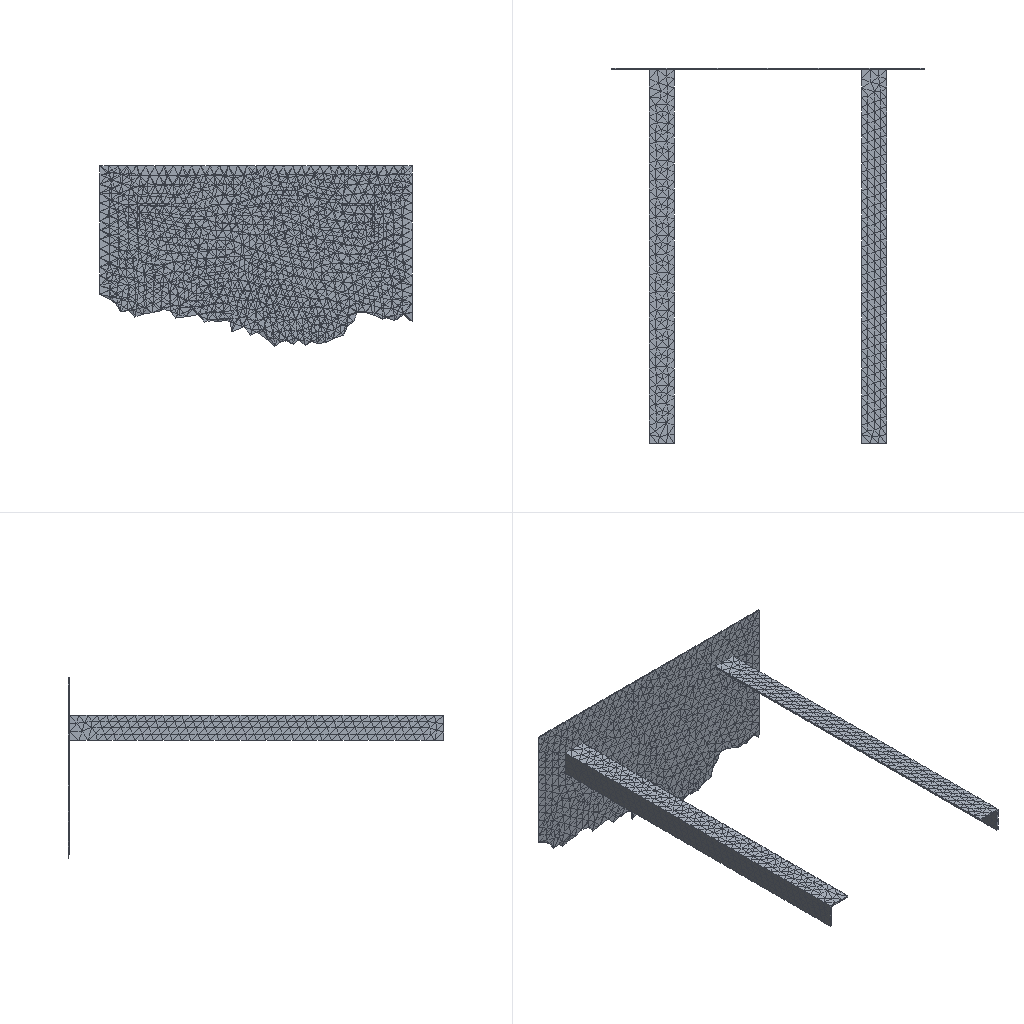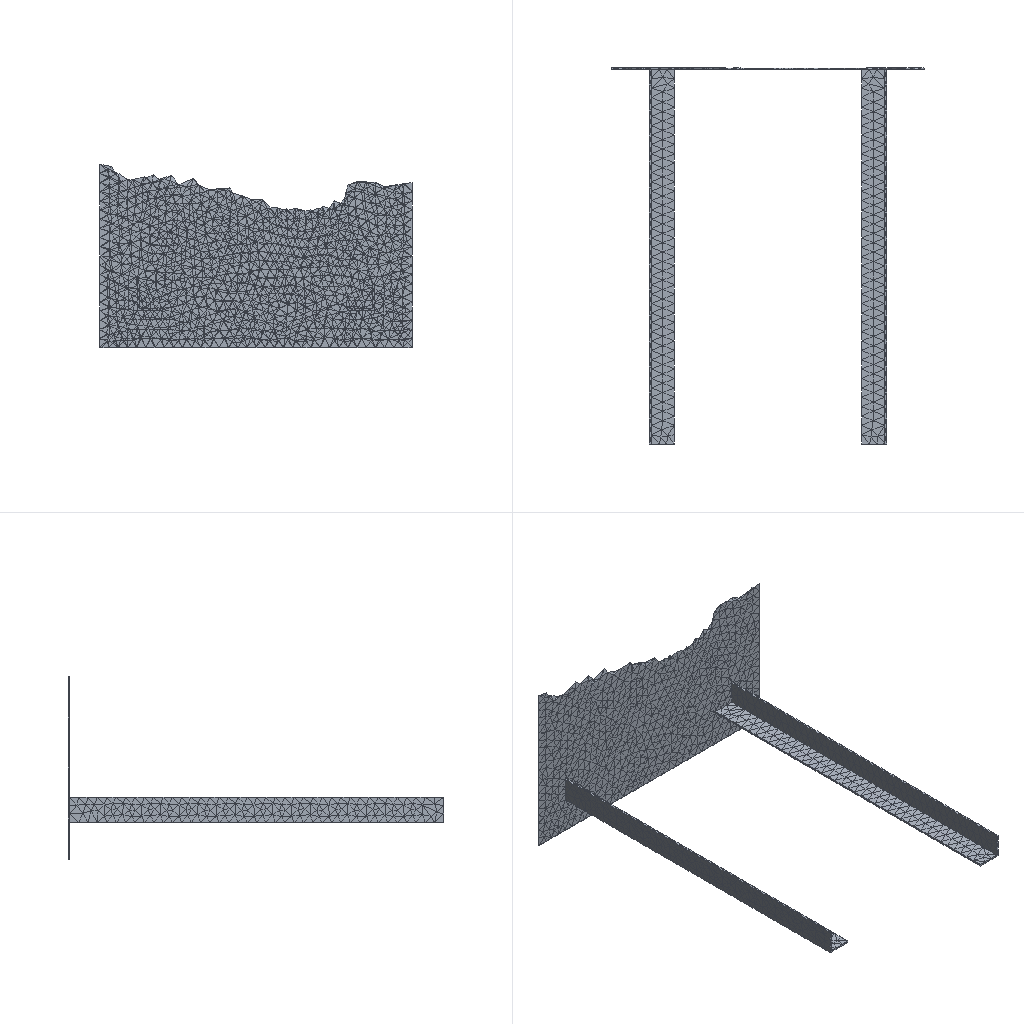Simulation study | ansys mapdl
Set-up summary:
category,name,step,type,value,unit,region
solver,ansys_mapdl
solver,version,,,21.1
solver,version,,,21.1
solver,version,,,21.1
units,MPA,,stated
analysis,deck,,modal,modal
load_step,requested,,,1
analysis,nlgeom,,,False
mesh,nodes,,,27244
mesh,elements,,,12925
element_type,ANSYS 187 (type 1),,solid,12925
load,load commands in deck,,count,0
bc,support commands in deck,,count,1
named_set,_CM35_FIXEDSU,,component
named_set,_CONSTRAINEDNODES,,component
named_set,_FIXEDSU,,component
material,1,,in results
material,1,,in results
material,1,,in results
check,setup vs results,,match
Ansys APDL input file, long lists of numbers shortened:
/batch
/config,noeldb,1     ! force off writing results to database
*get,_wallstrt,active,,time,wall
! ANSYS input file written by Workbench version 2021 R1
! File used for geometry attach: D:\___\_____\____\__________________________________________..........____...........____\______\____\____.agdb
/title,wbnew--__ (A5)
! ****** Begin Custom Load Command Snippet ******
/COM, ACT Extensions:
/COM,     LSDYNA, 2021.1
/COM,
! ****** End   Custom Load Command Snippet ******
*DIM,_wb_ProjectScratch_dir,string,248
_wb_ProjectScratch_dir(1) = 'C:\_____\_____________\_______\_____\____\________________________\_______________\_______\_
*DIM,_wb_SolverFiles_dir,string,248
_wb_SolverFiles_dir(1) = 'C:\_____\_____________\_______\_____\____\________________________\___________\___\___\____\_
*DIM,_wb_userfiles_dir,string,248
_wb_userfiles_dir(1) = 'C:\_____\_____________\_______\_____\____\________________________\___________\__________\_
/com,--- Data in consistent NMM units. See Solving Units in the help system for more information.
/units,MPA
/nopr
/wb,file,start              !  signify a WB generated input file
/prep7
! Turn off shape checking because checks already performed inside WB mesher.
! See help system for more information.
SHPP,OFF,,NOWARN
/nolist
etcon,set             ! allow ANSYS to choose best KEYOP's for 180x elements, resets any applicable keyopt to MAPDL defaults
/com,*********** Nodes for the whole assembly ***********
nblock,3,,29968
(1i9,3e20.9e3)
        1    -1.500000000E+02     0.000000000E+00    -1.900000000E+02
! (27243 more lines like these left out)
-1
/wb,elem,start            !  set before creation of elements
/com,*********** Elements for Body 1 "__" ***********
et,1,187
eblock,19,solid,,12925
(19i9)
        1        1        1        1        0        0        0        0       10        0        1      319      450     4260     4301     6715     7497     6717     6718
! (25849 more lines like these left out)
-1
/wb,elem,end               !  done creating elements
/com,*********** Send User Defined Coordinate System(s) ***********
csys,0
toffst,273.15,  ! Temperature offset from absolute zero
/com,*********** Set Reference Temperature ***********
tref,22.
/wb,mat,start              !  starting to send materials
/com,*********** Send Materials ***********
Temperature = 'TEMP' ! Temperature
MP,DENS,1,7.85e-09,	! tonne mm^-3
MP,ALPX,1,1.2e-05,	! C^-1
MP,C,1,434000000,	! mm^2 s^-2 C^-1
MP,KXX,1,60.5,	! tonne mm s^-3 C^-1
MP,RSVX,1,0.00017,	! ohm mm
MP,EX,1,200000,	! tonne s^-2 mm^-1
MP,NUXY,1,0.3,
MP,MURX,1,10000,
/wb,mat,end                !  done sending materials
!************************* Model Summary ********************
!__, Structural steel, matid, 1
!************************* End Model Summary ********************
! get the diagonal of the bounding box. Needed later for other things
*get,_xmin,node,,mnloc,x
*get,_ymin,node,,mnloc,y
*get,_zmin,node,,mnloc,z
*get,_xmax,node,,mxloc,x
*get,_ymax,node,,mxloc,y
*get,_zmax,node,,mxloc,z
_ASMDIAG=(_xmax-_xmin)*(_xmax-_xmin)+(_ymax-_ymin)*(_ymax-_ymin)+(_zmax-_zmin)*(_zmax-_zmin)
_ASMDIAG=SQRT(_ASMDIAG)
/wb,contact,start          !  starting to send contact
/wb,contact,end            !  done creating contacts
/golist
/wb,load,start             !  starting to send loads
CMBLOCK,_CM35_FIXEDSU,NODE,      156
(8i10)
         5        45        46        47        90        91        92       133
! (19 more lines like these left out)
/com,*********** Fixed Supports ***********
CMBLOCK,_FIXEDSU,NODE,      156
(8i10)
         5        45        46        47        90        91        92       133
! (19 more lines like these left out)
cmsel,s,_FIXEDSU
d,all,all
nsel,all
/gst,on,on
fini
*get,_numnode,node,0,count
*get,_numelem,elem,0,count
*get, _MAXELEMNUM, elem, 0, NUM, MAX
*get, _MAXNODENUM, node, 0, NUM, MAX
*get, _MAXELEMTYPE, etyp, 0, NUM, MAX
*get, _MAXREALCONST, real, 0, NUM, MAX
/go
/wb,load,end               !  done creating loads
/com,--- Number of total nodes = %_numnode%
/com,--- Number of contact elements = 0
/com,--- Number of spring elements = 0
/com,--- Number of bearing elements = 0
/com,--- Number of solid elements = 12925
/com,--- Number of condensed parts = 0
/com,--- Number of total elements = %_numelem%
*get,_wallbsol,active,,time,wall
/solu
antype,2                   ! modal analysis
_thickRatio=  0     ! Ratio of thick parts in the model
modopt,lanb,6
outres,erase
outres,all,none
outres,nsol,all
outres,etmp,all
outres,strs,all
outres,epel,all
outres,eppl,all
outres,rsol,all
nsel,s,d,U
nsel,a,d,ROT
esln
cm,_ConstrainedNodes,elem  ! -- reduced set with only constrained nodes
nsel,all
esel,all
outres,nload,all,_ConstrainedNodes  !-- reduced set with only constrained nodes
mxpand,,,,yes,,yes             ! expand requested element results, and write them to file.mode
dmpopt,esav,no
dmpopt,emat,no
dmpopt,full,no
! *********** WB SOLVE COMMAND ***********
! check interactive state
*get,ANSINTER_,active,,int
*if,ANSINTER_,ne,0,then
/eof
*endif
solve
/com *************** Write FE CONNECTORS *********
CEWRITE,file,ce,,INTE
*get,_nmodalsolproc,active,0,numcpu
fini
save,file,db
/nopr
*get,_numnode,node,0,count
*get,_numelem,elem,0,count
*get, _MAXELEMNUM, elem, 0, NUM, MAX
*get, _MAXNODENUM, node, 0, NUM, MAX,,,INTERNAL
*get, _MAXELEMTYPE, etyp, 0, NUM, MAX
*get, _MAXREALCONST, real, 0, NUM, MAX
/gopr
*get,_wallasol,active,,time,wall
/post1
/nopr
*dim,_direction,CHAR,6,1
_direction(1) = 'X'
_direction(2) = 'Y'
_direction(3) = 'Z'
_direction(4) = 'ROTX'
_direction(5) = 'ROTY'
_direction(6) = 'ROTZ'
*get,_lastLS,active,0,set,LSTP
*get,_beginset,active,0,set,nset,first,_lastLS
*get,_endset,active,0,set,nset,last,_lastLS
_nummodes = 0
*if,_endset,gt,0,then
_nummodes = _endset - _beginset + 1
*endif
*do,i_mode,1,_nummodes
   *do,j_component,1,6
			*get,PFACT_%i_mode%_%j_component%,MODE,%i_mode%,PFACT,,DIREC,_direction(%j_component%)
   *enddo
*enddo
*dim,_tmdirection,CHAR,6,1
_tmdirection(1) = 'X'
_tmdirection(2) = 'Y'
_tmdirection(3) = 'Z'
_tmdirection(4) = 'X'
_tmdirection(5) = 'Y'
_tmdirection(6) = 'Z'
*do,j_component,1,6
    *if,j_component,gt,3,then
        *get,TOTALMASS_%j_component%,ELEM,0,IOR,_tmdirection(%j_component%)
    *else
        *get,TOTALMASS_%j_component%,ELEM,0,MTOT,_tmdirection(%j_component%)
    *endif
*enddo
/gopr
xmlo,ENCODING,ISO-8859-1
xmlo,parm
/xml,parm,xml
fini
/gopr
*get,_walldone,active,,time,wall
_preptime=(_wallbsol-_wallstrt)*3600
_solvtime=(_wallasol-_wallbsol)*3600
_posttime=(_walldone-_wallasol)*3600
_totaltim=(_walldone-_wallstrt)*3600
*get,_dlbratio,active,0,solu,dlbr
*get,_combtime,active,0,solu,comb
/com,--- Total number of nodes = %_numnode%
/com,--- Total number of elements = %_numelem%
/com,--- Element load balance ratio = %_dlbratio%
/com,--- Time to combine distributed files = %_combtime%
/wb,file,end               ! done with WB generated input
Results summary:
result,analysis,,,modal
result,last_loadstep,,,1
result,primary field,,,displacement
result,reaction total,6,FX,-60.302,N
result,reaction total,6,FY,-2046.952,N
result,reaction total,6,FZ,69.841,N
result,analysis,,,modal
result,last_loadstep,,,1
result,primary field,,,displacement
result,reaction total,6,FX,-78.118,N
result,reaction total,6,FY,1965.552,N
result,reaction total,6,FZ,-55.7,N
result,analysis,,,modal
result,last_loadstep,,,1
result,primary field,,,displacement
result,reaction total,6,FX,-138.42,N
result,reaction total,6,FY,-81.4,N
result,reaction total,6,FZ,14.142,N